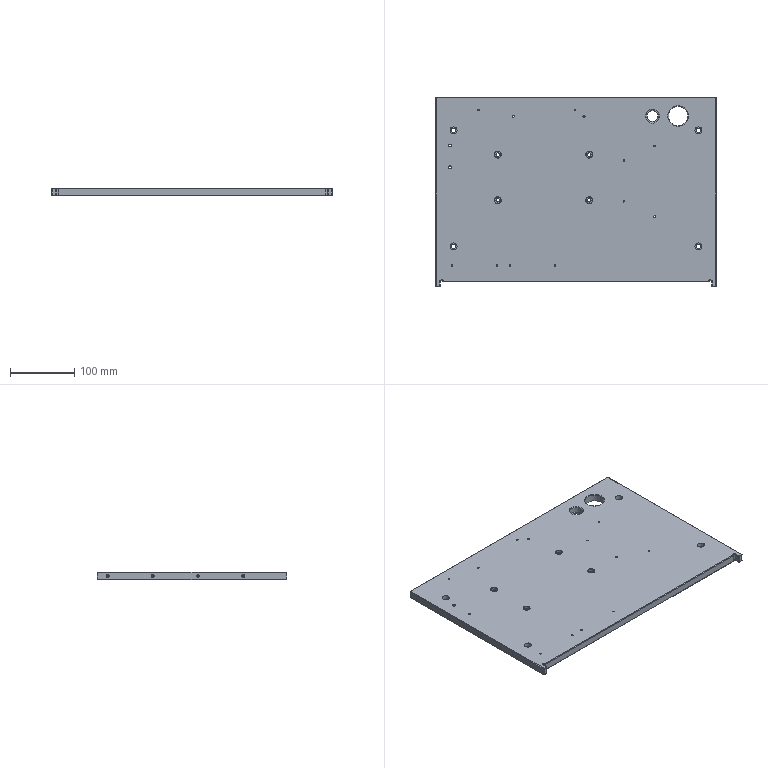Part | 1 solid | 124 faces | box 435 x 294.7 x 12 mm | volume 1477822 mm3 | cylinder 66 | cone 21 | plane 19 | sphere 12 | torus 6 | commonest cylinder face diameters 2 x22 3.3 x11 2.5 x10 5.5 x4 6.6 x4 10 x4